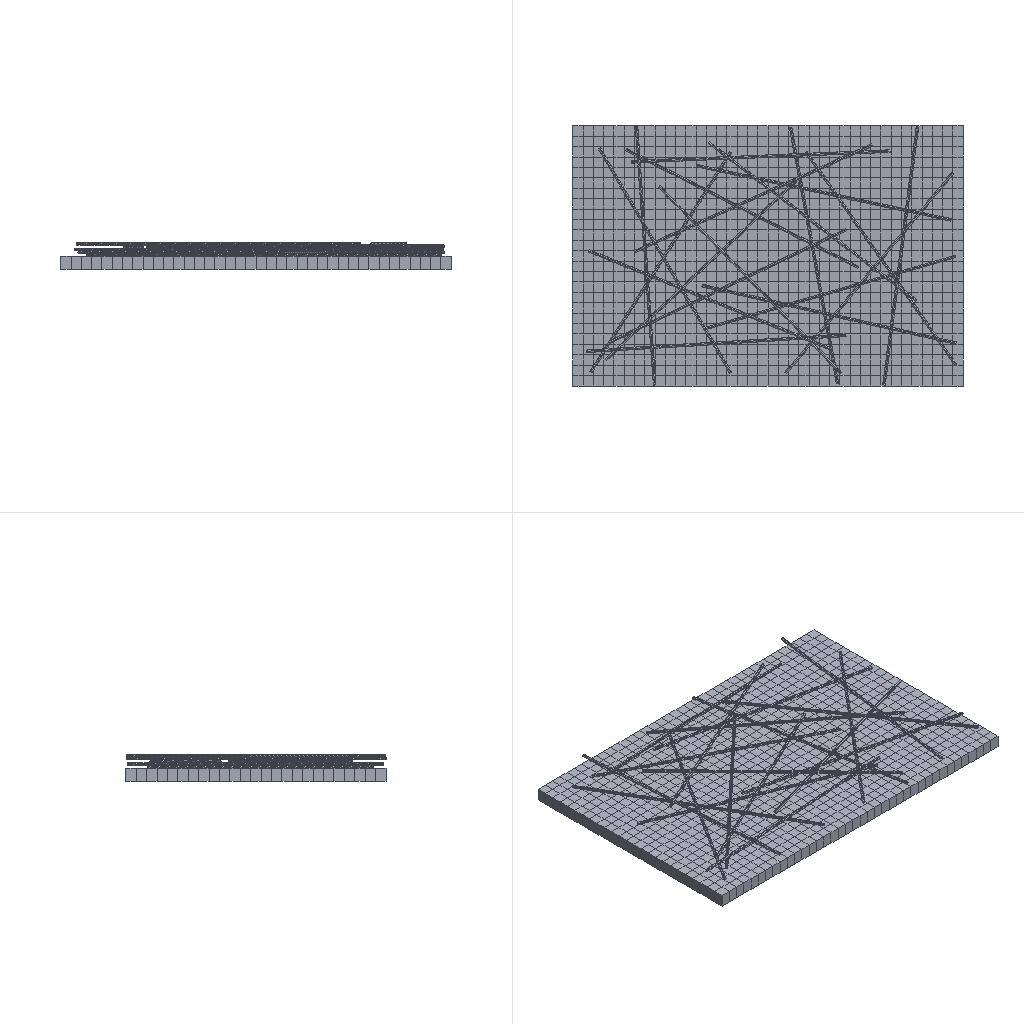Simulation study | abaqus
Set-up summary:
category,name,step,type,value,unit,region
solver,abaqus
solver,version,,,Abaqus/Explicit 2020
units,not stated in the deck,,not stated
analysis,deck,,transient,transient
load_step,Step-1,Step-1,transient
load_step,Step-2,Step-2,transient
load_step,requested,,,2
mesh,nodes,,,6474
mesh,elements,,,2850
element_type,C3D8R,,solid,2850
load,load commands in deck,,count,3
bc,support commands in deck,,count,18
material,JITI,,in results
material,MATERIAL-1,,in results
check,setup vs results,,match,"per instance, exact: element labels, types and connectivity; labels of the nodes the elements use; coordinates of those nodes at SINGLE_PRECISION in 19 of 20 instance(s)"
Abaqus input file, long lists of numbers shortened:
*Heading
** Job name: Job-1 Model name: Model-1
** Generated by: Abaqus/CAE 2020
*Preprint, echo=NO, model=NO, history=NO, contact=NO
**
** PARTS
**
*Part, name=P1111-1
*End Part
**
*Part, name=P1111-2
*End Part
**
*Part, name=P1111-3
*End Part
**
*Part, name=P1111-4
*End Part
**
*Part, name=P1111-5
*End Part
**
*Part, name=P1111-6
*End Part
**
*Part, name=P1111-7
*End Part
**
*Part, name=P1111-8
*End Part
**
*Part, name=P1111-9
*End Part
**
*Part, name=P1111-10
*End Part
**
*Part, name=P1111-11
*End Part
**
*Part, name=P1111-12
*End Part
**
*Part, name=P1111-13
*End Part
**
*Part, name=P1111-14
*End Part
**
*Part, name=P1111-15
*End Part
**
*Part, name=P1111-16
*End Part
**
*Part, name=P1111-17
*End Part
**
*Part, name=P1111-18
*End Part
**
*Part, name=P1111-19
*End Part
**
*Part, name=P1111-20
*End Part
**
**
** ASSEMBLY
**
*Assembly, name=Assembly
**
*Instance, name=P1111-1-1, part=P1111-1
*Node
      1,  -42.19,   54.229,           0.
      2,  -42.19,   50.229,           0.
** (2026 more lines like these left out)
*Element, type=C3D8R
  1,   53,   54,   80,   79,    1,    2,   28,   27
  2,   54,   55,   81,   80,    2,    3,   29,   28
** (948 more lines like these left out)
*Nset, nset=Set-1, generate
    1,  2028,     1
*Elset, elset=Set-1, generate
   1,  950,    1
** Section: jiti
*Solid Section, elset=Set-1, material=jiti
,
*End Instance
**
*Instance, name=P1111-2-1, part=P1111-2
*Node
      1,  -31.669,   45.76,   5.139
      2,  -31.974,   45.582,   4.992
** (232 more lines like these left out)
*Element, type=C3D8R
  1,   1,   9,   3,   2,  10,  18,  12,  11
  2,   7,   6,   5,   9,  16,  15,  14,  18
** (98 more lines like these left out)
*Nset, nset=Set-1, generate
   1,  234,    1
*Elset, elset=Set-1, generate
   1,  100,    1
** Section: yuanzhu
*Solid Section, elset=Set-1, material=Material-1
,
*End Instance
**
*Instance, name=P1111-3-1, part=P1111-3
*Node
      1,   104.08,   35.777,   5.139
      2,    103.809,   36.004,   4.992
** (232 more lines like these left out)
*Element, type=C3D8R
  1,   2,   1,   8,   9,  11,  10,  17,  18
  2,   2,   9,   4,   3,  11,  18,  13,  12
** (98 more lines like these left out)
*Nset, nset=Set-1, generate
   1,  234,    1
*Elset, elset=Set-1, generate
   1,  100,    1
** Section: yuanzhu
*Solid Section, elset=Set-1, material=Material-1
,
*End Instance
**
*Instance, name=P1111-4-1, part=P1111-4
*Node
      1,  -21.552,   45.409,   5.139
      2,  -21.712,   45.094,   4.992
** (232 more lines like these left out)
*Element, type=C3D8R
  1,   6,   9,   8,   7,  15,  18,  17,  16
  2,   4,   3,   2,   9,  13,  12,  11,  18
** (98 more lines like these left out)
*Nset, nset=Set-1, generate
   1,  234,    1
*Elset, elset=Set-1, generate
   1,  100,    1
** Section: yuanzhu
*Solid Section, elset=Set-1, material=Material-1
,
*End Instance
**
*Instance, name=P1111-5-1, part=P1111-5
*Node
      1,   -35.497,  -40.087,   6.265
      2,  -35.199,  -40.277,   6.118
** (232 more lines like these left out)
*Element, type=C3D8R
  1,   4,   9,   6,   5,  13,  18,  15,  14
  2,   8,   7,   6,   9,  17,  16,  15,  18
** (98 more lines like these left out)
*Nset, nset=Set-1, generate
   1,  234,    1
*Elset, elset=Set-1, generate
   1,  100,    1
** Section: yuanzhu
*Solid Section, elset=Set-1, material=Material-1
,
*End Instance
**
*Instance, name=P1111-6-1, part=P1111-6
*Node
      1,   104.726,  -37.897,   6.265
      2,   105.015,  -37.693,   6.118
** (232 more lines like these left out)
*Element, type=C3D8R
  1,   6,   9,   8,   7,  15,  18,  17,  16
  2,   6,   5,   4,   9,  15,  14,  13,  18
** (98 more lines like these left out)
*Nset, nset=Set-1, generate
   1,  234,    1
*Elset, elset=Set-1, generate
   1,  100,    1
** Section: yuanzhu
*Solid Section, elset=Set-1, material=Material-1
,
*End Instance
**
*Instance, name=P1111-7-1, part=P1111-7
*Node
      1,   59.185,  -44.893,   6.265
      2,   59.533,  -44.83,   6.118
** (232 more lines like these left out)
*Element, type=C3D8R
  1,   4,   3,   2,   9,  13,  12,  11,  18
  2,   4,   9,   6,   5,  13,  18,  15,  14
** (98 more lines like these left out)
*Nset, nset=Set-1, generate
   1,  234,    1
*Elset, elset=Set-1, generate
   1,  100,    1
** Section: yuanzhu
*Solid Section, elset=Set-1, material=Material-1
,
*End Instance
**
*Instance, name=P1111-8-1, part=P1111-8
*Node
      1,  -29.698,  -35.221,   6.303
      2,   -29.456,  -35.479,    6.156
** (232 more lines like these left out)
*Element, type=C3D8R
  1,   8,   7,   6,   9,  17,  16,  15,  18
  2,   8,   9,   2,   1,  17,  18,  11,  10
** (98 more lines like these left out)
*Nset, nset=Set-1, generate
   1,  234,    1
*Elset, elset=Set-1, generate
   1,  100,    1
** Section: yuanzhu
*Solid Section, elset=Set-1, material=Material-1
,
*End Instance
**
*Instance, name=P1111-9-1, part=P1111-9
*Node
      1,  -37.063,  -32.075,   7.313
      2,  -37.041,  -32.428,   7.166
** (232 more lines like these left out)
*Element, type=C3D8R
  1,   6,   9,   8,   7,  15,  18,  17,  16
  2,   4,   3,   2,   9,  13,  12,  11,  18
** (98 more lines like these left out)
*Nset, nset=Set-1, generate
   1,  234,    1
*Elset, elset=Set-1, generate
   1,  100,    1
** Section: yuanzhu
*Solid Section, elset=Set-1, material=Material-1
,
*End Instance
**
*Instance, name=P1111-10-1, part=P1111-10
*Node
      1,  -27.663,  -28.386,   7.313
      2,  -27.511,  -28.705,   7.166
** (232 more lines like these left out)
*Element, type=C3D8R
  1,   2,   1,   8,   9,  11,  10,  17,  18
  2,   4,   9,   6,   5,  13,  18,  15,  14
** (98 more lines like these left out)
*Nset, nset=Set-1, generate
   1,  234,    1
*Elset, elset=Set-1, generate
   1,  100,    1
** Section: yuanzhu
*Solid Section, elset=Set-1, material=Material-1
,
*End Instance
**
*Instance, name=P1111-11-1, part=P1111-11
*Node
      1,   5.398,   39.306,   7.313
      2,   5.324,   38.96,   7.166
** (232 more lines like these left out)
*Element, type=C3D8R
  1,   6,   9,   8,   7,  15,  18,  17,  16
  2,   8,   9,   2,   1,  17,  18,  11,  10
** (98 more lines like these left out)
*Nset, nset=Set-1, generate
   1,  234,    1
*Elset, elset=Set-1, generate
   1,  100,    1
** Section: yuanzhu
*Solid Section, elset=Set-1, material=Material-1
,
*End Instance
**
*Instance, name=P1111-12-1, part=P1111-12
*Node
      1,   7.535,  -6.803,   8.533
      2,   7.456,  -7.148,    8.386
** (232 more lines like these left out)
*Element, type=C3D8R
  1,   5,   9,   7,   6,  14,  18,  16,  15
  2,   1,   8,   7,   9,  10,  17,  16,  18
** (98 more lines like these left out)
*Nset, nset=Set-1, generate
   1,  234,    1
*Elset, elset=Set-1, generate
   1,  100,    1
** Section: yuanzhu
*Solid Section, elset=Set-1, material=Material-1
,
*End Instance
**
*Instance, name=P1111-13-1, part=P1111-13
*Node
      1,  -8.713,   31.118,   8.404
      2,  -8.966,    30.871,   8.258
** (232 more lines like these left out)
*Element, type=C3D8R
  1,   4,   9,   6,   5,  13,  18,  15,  14
  2,   8,   9,   2,   1,  17,  18,  11,  10
** (98 more lines like these left out)
*Nset, nset=Set-1, generate
   1,  234,    1
*Elset, elset=Set-1, generate
   1,  100,    1
** Section: yuanzhu
*Solid Section, elset=Set-1, material=Material-1
,
*End Instance
**
*Instance, name=P1111-14-1, part=P1111-14
*Node
      1,   90.585,   53.756,   9.437
      2,   90.235,   53.802,   9.29
** (232 more lines like these left out)
*Element, type=C3D8R
  1,   5,   9,   7,   6,  14,  18,  16,  15
  2,   1,   9,   3,   2,  10,  18,  12,  11
** (98 more lines like these left out)
*Nset, nset=Set-1, generate
   1,  234,    1
*Elset, elset=Set-1, generate
   1,  100,    1
** Section: yuanzhu
*Solid Section, elset=Set-1, material=Material-1
,
*End Instance
**
*Instance, name=P1111-15-1, part=P1111-15
*Node
      1,  -17.369,   53.979,   8.404
      2,  -17.722,    53.955,   8.258
** (232 more lines like these left out)
*Element, type=C3D8R
  1,   7,   6,   5,   9,  16,  15,  14,  18
  2,   5,   4,   3,   9,  14,  13,  12,  18
** (98 more lines like these left out)
*Nset, nset=Set-1, generate
   1,  234,    1
*Elset, elset=Set-1, generate
   1,  100,    1
** Section: yuanzhu
*Solid Section, elset=Set-1, material=Material-1
,
*End Instance
**
*Instance, name=P1111-16-1, part=P1111-16
*Node
      1,   10.313,   47.989,   8.404
      2,   10.099,   47.707,   8.258
** (232 more lines like these left out)
*Element, type=C3D8R
  1,   1,   9,   3,   2,  10,  18,  12,  11
  2,   7,   6,   5,   9,  16,  15,  14,  18
** (98 more lines like these left out)
*Nset, nset=Set-1, generate
   1,  234,    1
*Elset, elset=Set-1, generate
   1,  100,    1
** Section: yuanzhu
*Solid Section, elset=Set-1, material=Material-1
,
*End Instance
**
*Instance, name=P1111-17-1, part=P1111-17
*Node
      1,  -35.913,   6.512,   9.437
      2,   -36.045,   6.185,   9.29
** (232 more lines like these left out)
*Element, type=C3D8R
  1,   5,   9,   7,   6,  14,  18,  16,  15
  2,   5,   4,   3,   9,  14,  13,  12,  18
** (98 more lines like these left out)
*Nset, nset=Set-1, generate
   1,  234,    1
*Elset, elset=Set-1, generate
   1,  100,    1
** Section: yuanzhu
*Solid Section, elset=Set-1, material=Material-1
,
*End Instance
**
*Instance, name=P1111-18-1, part=P1111-18
*Node
      1,  -18.626,   6.193,   9.437
      2,  -18.481,   5.871,   9.29
** (232 more lines like these left out)
*Element, type=C3D8R
  1,   7,   6,   5,   9,  16,  15,  14,  18
  2,   1,   8,   7,   9,  10,  17,  16,  18
** (98 more lines like these left out)
*Nset, nset=Set-1, generate
   1,  234,    1
*Elset, elset=Set-1, generate
   1,  100,    1
** Section: yuanzhu
*Solid Section, elset=Set-1, material=Material-1
,
*End Instance
**
*Instance, name=P1111-19-1, part=P1111-19
*Node
      1,  -19.828,   40.731,   7.313
      2,  -19.814,   40.378,   7.166
** (232 more lines like these left out)
*Element, type=C3D8R
  1,   1,   9,   3,   2,  10,  18,  12,  11
  2,   7,   6,   5,   9,  16,  15,  14,  18
** (98 more lines like these left out)
*Nset, nset=Set-1, generate
   1,  234,    1
*Elset, elset=Set-1, generate
   1,  100,    1
** Section: yuanzhu
*Solid Section, elset=Set-1, material=Material-1
,
*End Instance
**
*Instance, name=P1111-20-1, part=P1111-20
*Node
      1,   8.641,  -23.322,   7.313
      2,   8.739,   -23.661,   7.166
** (232 more lines like these left out)
*Element, type=C3D8R
  1,   2,   1,   8,   9,  11,  10,  17,  18
  2,   4,   9,   6,   5,  13,  18,  15,  14
** (98 more lines like these left out)
*Nset, nset=Set-1, generate
   1,  234,    1
*Elset, elset=Set-1, generate
   1,  100,    1
** Section: yuanzhu
*Solid Section, elset=Set-1, material=Material-1
,
*End Instance
**
*Nset, nset=Set-1, instance=P1111-2-1, generate
   1,  234,    1
*Nset, nset=Set-1, instance=P1111-3-1, generate
   1,  234,    1
*Nset, nset=Set-1, instance=P1111-4-1, generate
   1,  234,    1
*Nset, nset=Set-1, instance=P1111-8-1, generate
   1,  234,    1
*Nset, nset=Set-1, instance=P1111-16-1, generate
   1,  234,    1
*Nset, nset=Set-1, instance=P1111-12-1, generate
   1,  234,    1
*Nset, nset=Set-1, instance=P1111-20-1, generate
   1,  234,    1
*Nset, nset=Set-1, instance=P1111-6-1, generate
   1,  234,    1
*Nset, nset=Set-1, instance=P1111-10-1, generate
   1,  234,    1
*Nset, nset=Set-1, instance=P1111-18-1, generate
   1,  234,    1
*Nset, nset=Set-1, instance=P1111-14-1, generate
   1,  234,    1
*Nset, nset=Set-1, instance=P1111-5-1, generate
   1,  234,    1
*Nset, nset=Set-1, instance=P1111-9-1, generate
   1,  234,    1
*Nset, nset=Set-1, instance=P1111-17-1, generate
   1,  234,    1
*Nset, nset=Set-1, instance=P1111-13-1, generate
   1,  234,    1
*Nset, nset=Set-1, instance=P1111-7-1, generate
   1,  234,    1
*Nset, nset=Set-1, instance=P1111-11-1, generate
   1,  234,    1
*Nset, nset=Set-1, instance=P1111-19-1, generate
   1,  234,    1
*Nset, nset=Set-1, instance=P1111-15-1, generate
   1,  234,    1
*Elset, elset=Set-1, instance=P1111-2-1, generate
   1,  100,    1
*Elset, elset=Set-1, instance=P1111-3-1, generate
   1,  100,    1
*Elset, elset=Set-1, instance=P1111-4-1, generate
   1,  100,    1
*Elset, elset=Set-1, instance=P1111-8-1, generate
   1,  100,    1
*Elset, elset=Set-1, instance=P1111-16-1, generate
   1,  100,    1
*Elset, elset=Set-1, instance=P1111-12-1, generate
   1,  100,    1
*Elset, elset=Set-1, instance=P1111-20-1, generate
   1,  100,    1
*Elset, elset=Set-1, instance=P1111-6-1, generate
   1,  100,    1
*Elset, elset=Set-1, instance=P1111-10-1, generate
   1,  100,    1
*Elset, elset=Set-1, instance=P1111-18-1, generate
   1,  100,    1
*Elset, elset=Set-1, instance=P1111-14-1, generate
   1,  100,    1
*Elset, elset=Set-1, instance=P1111-5-1, generate
   1,  100,    1
*Elset, elset=Set-1, instance=P1111-9-1, generate
   1,  100,    1
*Elset, elset=Set-1, instance=P1111-17-1, generate
   1,  100,    1
*Elset, elset=Set-1, instance=P1111-13-1, generate
   1,  100,    1
*Elset, elset=Set-1, instance=P1111-7-1, generate
   1,  100,    1
*Elset, elset=Set-1, instance=P1111-11-1, generate
   1,  100,    1
*Elset, elset=Set-1, instance=P1111-19-1, generate
   1,  100,    1
*Elset, elset=Set-1, instance=P1111-15-1, generate
   1,  100,    1
*Nset, nset=Set-2, instance=P1111-1-1, generate
  1,  52,   1
*Elset, elset=Set-2, instance=P1111-1-1, generate
  1,  25,   1
*Nset, nset=Set-3, instance=P1111-1-1, generate
 1977,  2028,     1
*Elset, elset=Set-3, instance=P1111-1-1, generate
 926,  950,    1
*Nset, nset=Set-4, instance=P1111-1-1
    1,    2,    3,    4,    5,    6,    7,    8,    9,   10,   11,   12,   13,   14,   15,   16
   17,   18,   19,   20,   21,   22,   23,   24,   25,   26,   53,   54,   55,   56,   57,   58
** (62 more lines like these left out)
*Elset, elset=Set-4, instance=P1111-1-1, generate
   1,  950,    1
*Elset, elset=_m_Surf-1_S5, internal, instance=P1111-2-1, generate
  1,  97,   4
*Elset, elset=_m_Surf-1_S5, internal, instance=P1111-3-1
  2,  3,  6,  7, 10, 11, 14, 15, 18, 19, 22, 23, 26, 27, 30, 31
 34, 35, 38, 39, 42, 43, 46, 47, 50, 51, 54, 55, 58, 59, 62, 63
** (2 more lines like these left out)
*Elset, elset=_m_Surf-1_S5, internal, instance=P1111-4-1
   1,   3,   4,   5,   7,   8,   9,  11,  12,  13,  15,  16,  17,  19,  20,  21
  23,  24,  25,  27,  28,  29,  31,  32,  33,  35,  36,  37,  39,  40,  41,  43
** (3 more lines like these left out)
*Elset, elset=_m_Surf-1_S5, internal, instance=P1111-8-1
   2,   3,   4,   6,   7,   8,  10,  11,  12,  14,  15,  16,  18,  19,  20,  22
  23,  24,  26,  27,  28,  30,  31,  32,  34,  35,  36,  38,  39,  40,  42,  43
** (3 more lines like these left out)
*Elset, elset=_m_Surf-1_S5, internal, instance=P1111-16-1, generate
  1,  99,   2
*Elset, elset=_m_Surf-1_S5, internal, instance=P1111-12-1
   1,   4,   5,   8,   9,  12,  13,  16,  17,  20,  21,  24,  25,  28,  29,  32
  33,  36,  37,  40,  41,  44,  45,  48,  49,  52,  53,  56,  57,  60,  61,  64
** (2 more lines like these left out)
*Elset, elset=_m_Surf-1_S5, internal, instance=P1111-20-1
  2,  3,  6,  7, 10, 11, 14, 15, 18, 19, 22, 23, 26, 27, 30, 31
 34, 35, 38, 39, 42, 43, 46, 47, 50, 51, 54, 55, 58, 59, 62, 63
** (2 more lines like these left out)
*Elset, elset=_m_Surf-1_S5, internal, instance=P1111-6-1
   1,   3,   4,   5,   7,   8,   9,  11,  12,  13,  15,  16,  17,  19,  20,  21
  23,  24,  25,  27,  28,  29,  31,  32,  33,  35,  36,  37,  39,  40,  41,  43
** (3 more lines like these left out)
*Elset, elset=_m_Surf-1_S5, internal, instance=P1111-10-1
  2,  3,  6,  7, 10, 11, 14, 15, 18, 19, 22, 23, 26, 27, 30, 31
 34, 35, 38, 39, 42, 43, 46, 47, 50, 51, 54, 55, 58, 59, 62, 63
** (2 more lines like these left out)
*Elset, elset=_m_Surf-1_S5, internal, instance=P1111-18-1, generate
  3,  99,   4
*Elset, elset=_m_Surf-1_S5, internal, instance=P1111-14-1
  1,  2,  3,  5,  6,  7,  9, 10, 11, 13, 14, 15, 17, 18, 19, 21
 22, 23, 25, 26, 27, 29, 30, 31, 33, 34, 35, 37, 38, 39, 41, 42
** (3 more lines like these left out)
*Elset, elset=_m_Surf-1_S5, internal, instance=P1111-5-1, generate
  1,  97,   4
*Elset, elset=_m_Surf-1_S5, internal, instance=P1111-9-1
   1,   3,   4,   5,   7,   8,   9,  11,  12,  13,  15,  16,  17,  19,  20,  21
  23,  24,  25,  27,  28,  29,  31,  32,  33,  35,  36,  37,  39,  40,  41,  43
** (3 more lines like these left out)
*Elset, elset=_m_Surf-1_S5, internal, instance=P1111-17-1
   1,   4,   5,   8,   9,  12,  13,  16,  17,  20,  21,  24,  25,  28,  29,  32
  33,  36,  37,  40,  41,  44,  45,  48,  49,  52,  53,  56,  57,  60,  61,  64
** (2 more lines like these left out)
*Elset, elset=_m_Surf-1_S5, internal, instance=P1111-13-1
  1,  2,  3,  5,  6,  7,  9, 10, 11, 13, 14, 15, 17, 18, 19, 21
 22, 23, 25, 26, 27, 29, 30, 31, 33, 34, 35, 37, 38, 39, 41, 42
** (3 more lines like these left out)
*Elset, elset=_m_Surf-1_S5, internal, instance=P1111-7-1, generate
  2,  98,   4
*Elset, elset=_m_Surf-1_S5, internal, instance=P1111-11-1, generate
   1,  100,    1
*Elset, elset=_m_Surf-1_S5, internal, instance=P1111-19-1, generate
  1,  99,   2
*Elset, elset=_m_Surf-1_S5, internal, instance=P1111-15-1, generate
   4,  100,    4
*Elset, elset=_m_Surf-1_S6, internal, instance=P1111-2-1, generate
  1,  97,   4
*Elset, elset=_m_Surf-1_S6, internal, instance=P1111-3-1
  2,  3,  6,  7, 10, 11, 14, 15, 18, 19, 22, 23, 26, 27, 30, 31
 34, 35, 38, 39, 42, 43, 46, 47, 50, 51, 54, 55, 58, 59, 62, 63
** (2 more lines like these left out)
*Elset, elset=_m_Surf-1_S6, internal, instance=P1111-4-1
   1,   3,   4,   5,   7,   8,   9,  11,  12,  13,  15,  16,  17,  19,  20,  21
  23,  24,  25,  27,  28,  29,  31,  32,  33,  35,  36,  37,  39,  40,  41,  43
** (3 more lines like these left out)
*Elset, elset=_m_Surf-1_S6, internal, instance=P1111-8-1
   2,   3,   4,   6,   7,   8,  10,  11,  12,  14,  15,  16,  18,  19,  20,  22
  23,  24,  26,  27,  28,  30,  31,  32,  34,  35,  36,  38,  39,  40,  42,  43
** (3 more lines like these left out)
*Elset, elset=_m_Surf-1_S6, internal, instance=P1111-16-1, generate
  1,  99,   2
*Elset, elset=_m_Surf-1_S6, internal, instance=P1111-12-1
   1,   4,   5,   8,   9,  12,  13,  16,  17,  20,  21,  24,  25,  28,  29,  32
  33,  36,  37,  40,  41,  44,  45,  48,  49,  52,  53,  56,  57,  60,  61,  64
** (2 more lines like these left out)
*Elset, elset=_m_Surf-1_S6, internal, instance=P1111-20-1
  2,  3,  6,  7, 10, 11, 14, 15, 18, 19, 22, 23, 26, 27, 30, 31
 34, 35, 38, 39, 42, 43, 46, 47, 50, 51, 54, 55, 58, 59, 62, 63
** (2 more lines like these left out)
*Elset, elset=_m_Surf-1_S6, internal, instance=P1111-6-1
   1,   3,   4,   5,   7,   8,   9,  11,  12,  13,  15,  16,  17,  19,  20,  21
  23,  24,  25,  27,  28,  29,  31,  32,  33,  35,  36,  37,  39,  40,  41,  43
** (3 more lines like these left out)
*Elset, elset=_m_Surf-1_S6, internal, instance=P1111-10-1
  2,  3,  6,  7, 10, 11, 14, 15, 18, 19, 22, 23, 26, 27, 30, 31
 34, 35, 38, 39, 42, 43, 46, 47, 50, 51, 54, 55, 58, 59, 62, 63
** (2 more lines like these left out)
*Elset, elset=_m_Surf-1_S6, internal, instance=P1111-18-1, generate
  3,  99,   4
*Elset, elset=_m_Surf-1_S6, internal, instance=P1111-14-1
  1,  2,  3,  5,  6,  7,  9, 10, 11, 13, 14, 15, 17, 18, 19, 21
 22, 23, 25, 26, 27, 29, 30, 31, 33, 34, 35, 37, 38, 39, 41, 42
** (3 more lines like these left out)
*Elset, elset=_m_Surf-1_S6, internal, instance=P1111-5-1, generate
  1,  97,   4
*Elset, elset=_m_Surf-1_S6, internal, instance=P1111-9-1
   1,   3,   4,   5,   7,   8,   9,  11,  12,  13,  15,  16,  17,  19,  20,  21
  23,  24,  25,  27,  28,  29,  31,  32,  33,  35,  36,  37,  39,  40,  41,  43
** (3 more lines like these left out)
*Elset, elset=_m_Surf-1_S6, internal, instance=P1111-17-1
   1,   4,   5,   8,   9,  12,  13,  16,  17,  20,  21,  24,  25,  28,  29,  32
  33,  36,  37,  40,  41,  44,  45,  48,  49,  52,  53,  56,  57,  60,  61,  64
** (2 more lines like these left out)
*Elset, elset=_m_Surf-1_S6, internal, instance=P1111-13-1
  1,  2,  3,  5,  6,  7,  9, 10, 11, 13, 14, 15, 17, 18, 19, 21
 22, 23, 25, 26, 27, 29, 30, 31, 33, 34, 35, 37, 38, 39, 41, 42
** (3 more lines like these left out)
*Elset, elset=_m_Surf-1_S6, internal, instance=P1111-7-1, generate
  2,  98,   4
*Elset, elset=_m_Surf-1_S6, internal, instance=P1111-11-1, generate
   1,  100,    1
*Elset, elset=_m_Surf-1_S6, internal, instance=P1111-19-1, generate
  1,  99,   2
*Elset, elset=_m_Surf-1_S6, internal, instance=P1111-15-1, generate
   4,  100,    4
*Elset, elset=_m_Surf-1_S3, internal, instance=P1111-2-1
   2,   3,   4,   6,   7,   8,  10,  11,  12,  14,  15,  16,  18,  19,  20,  22
  23,  24,  26,  27,  28,  30,  31,  32,  34,  35,  36,  38,  39,  40,  42,  43
** (3 more lines like these left out)
*Elset, elset=_m_Surf-1_S3, internal, instance=P1111-3-1
   1,   4,   5,   8,   9,  12,  13,  16,  17,  20,  21,  24,  25,  28,  29,  32
  33,  36,  37,  40,  41,  44,  45,  48,  49,  52,  53,  56,  57,  60,  61,  64
** (2 more lines like these left out)
*Elset, elset=_m_Surf-1_S3, internal, instance=P1111-4-1, generate
  2,  98,   4
*Elset, elset=_m_Surf-1_S3, internal, instance=P1111-8-1, generate
  1,  97,   4
*Elset, elset=_m_Surf-1_S3, internal, instance=P1111-16-1, generate
   2,  100,    2
*Elset, elset=_m_Surf-1_S3, internal, instance=P1111-12-1
  2,  3,  6,  7, 10, 11, 14, 15, 18, 19, 22, 23, 26, 27, 30, 31
 34, 35, 38, 39, 42, 43, 46, 47, 50, 51, 54, 55, 58, 59, 62, 63
** (2 more lines like these left out)
*Elset, elset=_m_Surf-1_S3, internal, instance=P1111-20-1
   1,   4,   5,   8,   9,  12,  13,  16,  17,  20,  21,  24,  25,  28,  29,  32
  33,  36,  37,  40,  41,  44,  45,  48,  49,  52,  53,  56,  57,  60,  61,  64
** (2 more lines like these left out)
*Elset, elset=_m_Surf-1_S3, internal, instance=P1111-6-1, generate
  2,  98,   4
*Elset, elset=_m_Surf-1_S3, internal, instance=P1111-10-1
   1,   4,   5,   8,   9,  12,  13,  16,  17,  20,  21,  24,  25,  28,  29,  32
  33,  36,  37,  40,  41,  44,  45,  48,  49,  52,  53,  56,  57,  60,  61,  64
** (2 more lines like these left out)
*Elset, elset=_m_Surf-1_S3, internal, instance=P1111-18-1
   1,   2,   4,   5,   6,   8,   9,  10,  12,  13,  14,  16,  17,  18,  20,  21
  22,  24,  25,  26,  28,  29,  30,  32,  33,  34,  36,  37,  38,  40,  41,  42
** (3 more lines like these left out)
*Elset, elset=_m_Surf-1_S3, internal, instance=P1111-14-1, generate
   4,  100,    4
*Elset, elset=_m_Surf-1_S3, internal, instance=P1111-5-1
   2,   3,   4,   6,   7,   8,  10,  11,  12,  14,  15,  16,  18,  19,  20,  22
  23,  24,  26,  27,  28,  30,  31,  32,  34,  35,  36,  38,  39,  40,  42,  43
** (3 more lines like these left out)
*Elset, elset=_m_Surf-1_S3, internal, instance=P1111-9-1, generate
  2,  98,   4
*Elset, elset=_m_Surf-1_S3, internal, instance=P1111-17-1
  2,  3,  6,  7, 10, 11, 14, 15, 18, 19, 22, 23, 26, 27, 30, 31
 34, 35, 38, 39, 42, 43, 46, 47, 50, 51, 54, 55, 58, 59, 62, 63
** (2 more lines like these left out)
*Elset, elset=_m_Surf-1_S3, internal, instance=P1111-13-1, generate
   4,  100,    4
*Elset, elset=_m_Surf-1_S3, internal, instance=P1111-7-1
   1,   3,   4,   5,   7,   8,   9,  11,  12,  13,  15,  16,  17,  19,  20,  21
  23,  24,  25,  27,  28,  29,  31,  32,  33,  35,  36,  37,  39,  40,  41,  43
** (3 more lines like these left out)
*Elset, elset=_m_Surf-1_S3, internal, instance=P1111-19-1, generate
   2,  100,    2
*Elset, elset=_m_Surf-1_S3, internal, instance=P1111-15-1
  1,  2,  3,  5,  6,  7,  9, 10, 11, 13, 14, 15, 17, 18, 19, 21
 22, 23, 25, 26, 27, 29, 30, 31, 33, 34, 35, 37, 38, 39, 41, 42
** (3 more lines like these left out)
*Elset, elset=_m_Surf-1_S4, internal, instance=P1111-2-1
   2,   3,   4,   6,   7,   8,  10,  11,  12,  14,  15,  16,  18,  19,  20,  22
  23,  24,  26,  27,  28,  30,  31,  32,  34,  35,  36,  38,  39,  40,  42,  43
** (3 more lines like these left out)
*Elset, elset=_m_Surf-1_S4, internal, instance=P1111-3-1
   1,   4,   5,   8,   9,  12,  13,  16,  17,  20,  21,  24,  25,  28,  29,  32
  33,  36,  37,  40,  41,  44,  45,  48,  49,  52,  53,  56,  57,  60,  61,  64
** (2 more lines like these left out)
*Elset, elset=_m_Surf-1_S4, internal, instance=P1111-4-1, generate
  2,  98,   4
*Elset, elset=_m_Surf-1_S4, internal, instance=P1111-8-1, generate
  1,  97,   4
*Elset, elset=_m_Surf-1_S4, internal, instance=P1111-16-1, generate
   2,  100,    2
*Elset, elset=_m_Surf-1_S4, internal, instance=P1111-12-1
  2,  3,  6,  7, 10, 11, 14, 15, 18, 19, 22, 23, 26, 27, 30, 31
 34, 35, 38, 39, 42, 43, 46, 47, 50, 51, 54, 55, 58, 59, 62, 63
** (2 more lines like these left out)
*Elset, elset=_m_Surf-1_S4, internal, instance=P1111-20-1
   1,   4,   5,   8,   9,  12,  13,  16,  17,  20,  21,  24,  25,  28,  29,  32
  33,  36,  37,  40,  41,  44,  45,  48,  49,  52,  53,  56,  57,  60,  61,  64
** (2 more lines like these left out)
*Elset, elset=_m_Surf-1_S4, internal, instance=P1111-6-1, generate
  2,  98,   4
*Elset, elset=_m_Surf-1_S4, internal, instance=P1111-10-1
   1,   4,   5,   8,   9,  12,  13,  16,  17,  20,  21,  24,  25,  28,  29,  32
  33,  36,  37,  40,  41,  44,  45,  48,  49,  52,  53,  56,  57,  60,  61,  64
** (2 more lines like these left out)
*Elset, elset=_m_Surf-1_S4, internal, instance=P1111-18-1
   1,   2,   4,   5,   6,   8,   9,  10,  12,  13,  14,  16,  17,  18,  20,  21
  22,  24,  25,  26,  28,  29,  30,  32,  33,  34,  36,  37,  38,  40,  41,  42
** (3 more lines like these left out)
*Elset, elset=_m_Surf-1_S4, internal, instance=P1111-14-1, generate
   4,  100,    4
*Elset, elset=_m_Surf-1_S4, internal, instance=P1111-5-1
   2,   3,   4,   6,   7,   8,  10,  11,  12,  14,  15,  16,  18,  19,  20,  22
  23,  24,  26,  27,  28,  30,  31,  32,  34,  35,  36,  38,  39,  40,  42,  43
** (3 more lines like these left out)
*Elset, elset=_m_Surf-1_S4, internal, instance=P1111-9-1, generate
  2,  98,   4
*Elset, elset=_m_Surf-1_S4, internal, instance=P1111-17-1
  2,  3,  6,  7, 10, 11, 14, 15, 18, 19, 22, 23, 26, 27, 30, 31
 34, 35, 38, 39, 42, 43, 46, 47, 50, 51, 54, 55, 58, 59, 62, 63
** (2 more lines like these left out)
*Elset, elset=_m_Surf-1_S4, internal, instance=P1111-13-1, generate
   4,  100,    4
*Elset, elset=_m_Surf-1_S4, internal, instance=P1111-7-1
   1,   3,   4,   5,   7,   8,   9,  11,  12,  13,  15,  16,  17,  19,  20,  21
  23,  24,  25,  27,  28,  29,  31,  32,  33,  35,  36,  37,  39,  40,  41,  43
** (3 more lines like these left out)
*Elset, elset=_m_Surf-1_S4, internal, instance=P1111-19-1, generate
   2,  100,    2
*Elset, elset=_m_Surf-1_S4, internal, instance=P1111-15-1
  1,  2,  3,  5,  6,  7,  9, 10, 11, 13, 14, 15, 17, 18, 19, 21
 22, 23, 25, 26, 27, 29, 30, 31, 33, 34, 35, 37, 38, 39, 41, 42
** (3 more lines like these left out)
*Elset, elset=_m_Surf-1_S2, internal, instance=P1111-2-1, generate
  97,  100,    1
*Elset, elset=_m_Surf-1_S2, internal, instance=P1111-3-1, generate
  97,  100,    1
*Elset, elset=_m_Surf-1_S2, internal, instance=P1111-4-1, generate
  97,  100,    1
*Elset, elset=_m_Surf-1_S2, internal, instance=P1111-8-1, generate
  97,  100,    1
*Elset, elset=_m_Surf-1_S2, internal, instance=P1111-16-1, generate
  97,  100,    1
*Elset, elset=_m_Surf-1_S2, internal, instance=P1111-12-1, generate
  97,  100,    1
*Elset, elset=_m_Surf-1_S2, internal, instance=P1111-20-1, generate
  97,  100,    1
*Elset, elset=_m_Surf-1_S2, internal, instance=P1111-6-1, generate
  97,  100,    1
*Elset, elset=_m_Surf-1_S2, internal, instance=P1111-10-1, generate
  97,  100,    1
*Elset, elset=_m_Surf-1_S2, internal, instance=P1111-18-1, generate
  97,  100,    1
*Elset, elset=_m_Surf-1_S2, internal, instance=P1111-14-1, generate
  97,  100,    1
*Elset, elset=_m_Surf-1_S2, internal, instance=P1111-5-1, generate
  97,  100,    1
*Elset, elset=_m_Surf-1_S2, internal, instance=P1111-9-1, generate
  97,  100,    1
*Elset, elset=_m_Surf-1_S2, internal, instance=P1111-17-1, generate
  97,  100,    1
*Elset, elset=_m_Surf-1_S2, internal, instance=P1111-13-1, generate
  97,  100,    1
*Elset, elset=_m_Surf-1_S2, internal, instance=P1111-7-1, generate
  97,  100,    1
*Elset, elset=_m_Surf-1_S2, internal, instance=P1111-11-1, generate
  97,  100,    1
*Elset, elset=_m_Surf-1_S2, internal, instance=P1111-19-1, generate
  97,  100,    1
*Elset, elset=_m_Surf-1_S2, internal, instance=P1111-15-1, generate
  97,  100,    1
*Elset, elset=_m_Surf-1_S1, internal, instance=P1111-2-1, generate
 1,  4,  1
*Elset, elset=_m_Surf-1_S1, internal, instance=P1111-3-1, generate
 1,  4,  1
*Elset, elset=_m_Surf-1_S1, internal, instance=P1111-4-1, generate
 1,  4,  1
*Elset, elset=_m_Surf-1_S1, internal, instance=P1111-8-1, generate
 1,  4,  1
*Elset, elset=_m_Surf-1_S1, internal, instance=P1111-16-1, generate
 1,  4,  1
*Elset, elset=_m_Surf-1_S1, internal, instance=P1111-12-1, generate
 1,  4,  1
*Elset, elset=_m_Surf-1_S1, internal, instance=P1111-20-1, generate
 1,  4,  1
*Elset, elset=_m_Surf-1_S1, internal, instance=P1111-6-1, generate
 1,  4,  1
*Elset, elset=_m_Surf-1_S1, internal, instance=P1111-10-1, generate
 1,  4,  1
*Elset, elset=_m_Surf-1_S1, internal, instance=P1111-18-1, generate
 1,  4,  1
*Elset, elset=_m_Surf-1_S1, internal, instance=P1111-14-1, generate
 1,  4,  1
*Elset, elset=_m_Surf-1_S1, internal, instance=P1111-5-1, generate
 1,  4,  1
*Elset, elset=_m_Surf-1_S1, internal, instance=P1111-9-1, generate
 1,  4,  1
*Elset, elset=_m_Surf-1_S1, internal, instance=P1111-17-1, generate
 1,  4,  1
*Elset, elset=_m_Surf-1_S1, internal, instance=P1111-13-1, generate
 1,  4,  1
*Elset, elset=_m_Surf-1_S1, internal, instance=P1111-7-1, generate
 1,  4,  1
*Elset, elset=_m_Surf-1_S1, internal, instance=P1111-11-1, generate
 1,  4,  1
*Elset, elset=_m_Surf-1_S1, internal, instance=P1111-19-1, generate
 1,  4,  1
*Elset, elset=_m_Surf-1_S1, internal, instance=P1111-15-1, generate
 1,  4,  1
*Surface, type=ELEMENT, name=m_Surf-1
_m_Surf-1_S5, S5
_m_Surf-1_S6, S6
_m_Surf-1_S4, S4
_m_Surf-1_S2, S2
_m_Surf-1_S3, S3
_m_Surf-1_S1, S1
*Elset, elset=_s_Surf-1_S5, internal, instance=P1111-1-1, generate
   1,  950,    1
*Surface, type=ELEMENT, name=s_Surf-1
_s_Surf-1_S5, S5
** Constraint: Constraint-1
*Tie, name=Constraint-1, adjust=yes
s_Surf-1, m_Surf-1
*End Assembly
*Amplitude, name=Amp-1
             0.,              0.,             0.1,              1.
**
** MATERIALS
**
*Material, name=Material-1
*Density
 1e-09,
*Elastic
500., 0.35
*Material, name=jiti
*Density
 2e-09,
*Elastic
10., 0.4
**
** INTERACTION PROPERTIES
**
*Surface Interaction, name=IntProp-1
*Friction
 0.2,
*Surface Behavior, pressure-overclosure=HARD
**
** INTERACTIONS
**
** Interaction: Int-1
*Contact, op=NEW
*Contact Inclusions, ALL EXTERIOR
*Contact Property Assignment
 ,  , IntProp-1
** ----------------------------------------------------------------
**
** STEP: Step-1
**
*Step, name=Step-1, nlgeom=YES
*Dynamic, Explicit
, 0.1
*Bulk Viscosity
0.06, 1.2
**
** BOUNDARY CONDITIONS
**
** Name: [REDACTED] : Displacement/rotation angle
*Boundary
Set-4, 1, 1
Set-4, 2, 2
Set-4, 3, 3
Set-4, 4, 4
Set-4, 5, 5
Set-4, 6, 6
**
** LOADS
**
** Name: Load-1   Type: Gravity
*Dload
Set-1, GRAV, 9800., 0., 0., -1.
**
** OUTPUT REQUESTS
**
*Restart, write, number interval=1, time marks=NO
**
** FIELD OUTPUT: F-Output-1
**
*Output, field
*Node Output
CF, RF, RM, RT, U, V
*Element Output, directions=YES
E, LE, MISES, MISESMAX, MISESONLY, PE, PEEQ, PEMAG, S, SF, SSAVG
*Contact Output
CDISP, CFORCE, CSTRESS
*Output, history, frequency=0
*End Step
** ----------------------------------------------------------------
**
** STEP: Step-2
**
*Step, name=Step-2, nlgeom=YES
*Dynamic, Explicit
, 0.1
*Bulk Viscosity
0.06, 1.2
** Mass Scaling: Semi-Automatic
**               Whole Model
*Fixed Mass Scaling, factor=50.
**
** BOUNDARY CONDITIONS
**
** Name: BC-1 Type: 位移/转角
*Boundary, op=NEW, amplitude=Amp-1
Set-2, 1, 1, -20.
Set-2, 2, 2
Set-2, 3, 3
Set-2, 4, 4
Set-2, 5, 5
Set-2, 6, 6
** Name: BC-1-Copy Type: 位移/转角
*Boundary, op=NEW, amplitude=Amp-1
Set-3, 1, 1, 20.
Set-3, 2, 2
Set-3, 3, 3
Set-3, 4, 4
Set-3, 5, 5
Set-3, 6, 6
** Name: [REDACTED] : Displacement/rotation angle
*Boundary, op=NEW
**
** OUTPUT REQUESTS
**
*Restart, write, number interval=1, time marks=NO
**
** FIELD OUTPUT: F-Output-1
**
*Output, field
*Node Output
CF, RF, RM, RT, U, V
*Element Output, directions=YES
E, LE, MISES, MISESMAX, MISESONLY, PE, PEEQ, PEMAG, S, SF, SSAVG
*Contact Output
CDISP, CFORCE, CSTRESS
*Output, history, frequency=0
*End Step
Results summary:
result,step,Step-1,completed,increments=293677 time=0.1/0.1
result,step,Step-2,completed,increments=49271 time=0.1/0.1
result,analysis,,,transient
result,last_loadstep,,,2
result,primary field,,,U
result,reaction total,,FX,-0.6603,model units
result,reaction total,,FY,-3.744,model units
result,reaction total,,FZ,-0.2338,model units